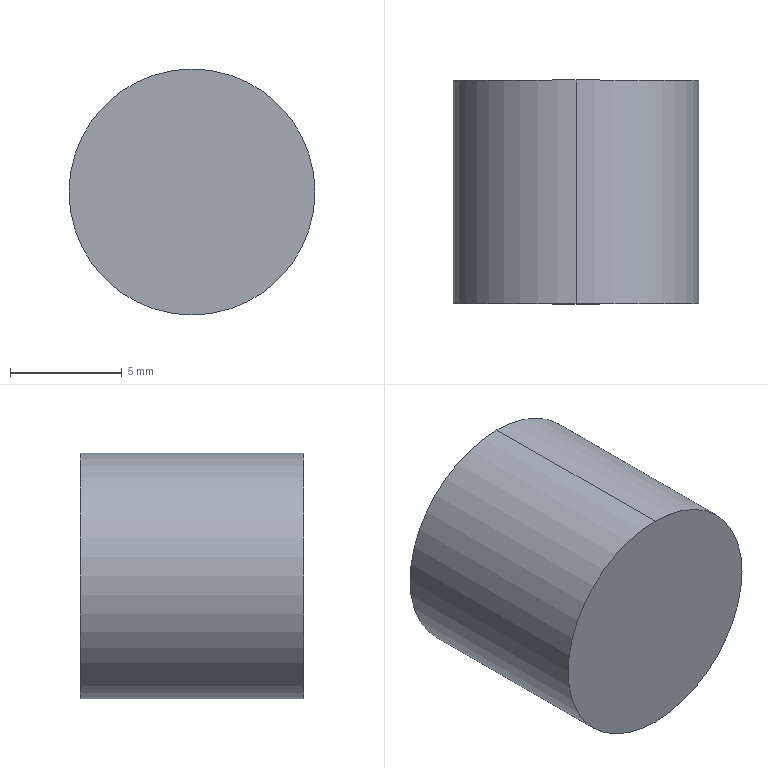Part | STEP file | OP10-129_seal pad M6 | 1 solid | 4 faces | box 11 x 10 x 11 mm | volume 950.332 mm3 | cylinder 2 | plane 2 | commonest cylinder face diameters 11 x2
STEP:
#1=CARTESIAN_POINT('',(0.,0.,0.));
#2=DIRECTION('',(0.,0.,1.));
#3=DIRECTION('',(1.,0.,0.));
#4=AXIS2_PLACEMENT_3D('',#1,#2,#3);
#5=CARTESIAN_POINT('',(0.,10.,5.5));
#6=VERTEX_POINT('',#5);
#7=CARTESIAN_POINT('',(0.,10.,-5.5));
#8=VERTEX_POINT('',#7);
#9=CARTESIAN_POINT('',(0.,10.,0.));
#10=DIRECTION('',(0.,1.,0.));
#11=DIRECTION('',(0.,0.,1.));
#12=AXIS2_PLACEMENT_3D('',#9,#10,#11);
#13=CIRCLE('',#12,5.5);
#14=CARTESIAN_POINT('',(0.,10.,0.));
#15=DIRECTION('',(0.,-1.,0.));
#16=DIRECTION('',(0.,0.,-1.));
#17=AXIS2_PLACEMENT_3D('',#14,#15,#16);
#18=CYLINDRICAL_SURFACE('',#17,5.5);
#19=CARTESIAN_POINT('',(3.142,0.));
#20=DIRECTION('',(-1.,0.));
#21=VECTOR('',#20,1.);
#22=LINE('',#19,#21);
#23=(GEOMETRIC_REPRESENTATION_CONTEXT(2)PARAMETRIC_REPRESENTATION_CONTEXT()REPRESENTATION_CONTEXT('',''));
#24=DEFINITIONAL_REPRESENTATION('',(#22),#23);
#25=PCURVE('',#18,#24);
#26=CARTESIAN_POINT('',(0.,10.,0.));
#27=DIRECTION('',(0.,1.,0.));
#28=DIRECTION('',(0.,0.,1.));
#29=AXIS2_PLACEMENT_3D('',#26,#27,#28);
#30=PLANE('',#29);
#31=CARTESIAN_POINT('',(0.,0.));
#32=DIRECTION('',(1.,0.));
#33=AXIS2_PLACEMENT_2D('',#31,#32);
#34=CIRCLE('',#33,5.5);
#35=(GEOMETRIC_REPRESENTATION_CONTEXT(2)PARAMETRIC_REPRESENTATION_CONTEXT()REPRESENTATION_CONTEXT('',''));
#36=DEFINITIONAL_REPRESENTATION('',(#34),#35);
#37=PCURVE('',#30,#36);
#38=SURFACE_CURVE('',#13,(#25,#37),.PCURVE_S1.);
#39=EDGE_CURVE('',#6,#8,#38,.T.);
#40=ORIENTED_EDGE('',*,*,#39,.F.);
#41=CARTESIAN_POINT('',(0.,0.,5.5));
#42=VERTEX_POINT('',#41);
#43=CARTESIAN_POINT('',(0.,10.,5.5));
#44=DIRECTION('',(0.,-1.,0.));
#45=VECTOR('',#44,1.);
#46=LINE('',#43,#45);
#47=CARTESIAN_POINT('',(3.142,0.));
#48=DIRECTION('',(0.,1.));
#49=VECTOR('',#48,1.);
#50=LINE('',#47,#49);
#51=(GEOMETRIC_REPRESENTATION_CONTEXT(2)PARAMETRIC_REPRESENTATION_CONTEXT()REPRESENTATION_CONTEXT('',''));
#52=DEFINITIONAL_REPRESENTATION('',(#50),#51);
#53=PCURVE('',#18,#52);
#54=CARTESIAN_POINT('',(0.,10.,0.));
#55=DIRECTION('',(0.,-1.,0.));
#56=DIRECTION('',(0.,0.,-1.));
#57=AXIS2_PLACEMENT_3D('',#54,#55,#56);
#58=CYLINDRICAL_SURFACE('',#57,5.5);
#59=CARTESIAN_POINT('',(3.142,0.));
#60=DIRECTION('',(0.,1.));
#61=VECTOR('',#60,1.);
#62=LINE('',#59,#61);
#63=(GEOMETRIC_REPRESENTATION_CONTEXT(2)PARAMETRIC_REPRESENTATION_CONTEXT()REPRESENTATION_CONTEXT('',''));
#64=DEFINITIONAL_REPRESENTATION('',(#62),#63);
#65=PCURVE('',#58,#64);
#66=SURFACE_CURVE('',#46,(#53,#65),.PCURVE_S1.);
#67=EDGE_CURVE('',#6,#42,#66,.T.);
#68=ORIENTED_EDGE('',*,*,#67,.T.);
#69=CARTESIAN_POINT('',(0.,0.,-5.5));
#70=VERTEX_POINT('',#69);
#71=CARTESIAN_POINT('',(0.,0.,0.));
#72=DIRECTION('',(0.,1.,0.));
#73=DIRECTION('',(0.,0.,1.));
#74=AXIS2_PLACEMENT_3D('',#71,#72,#73);
#75=CIRCLE('',#74,5.5);
#76=CARTESIAN_POINT('',(3.142,10.));
#77=DIRECTION('',(-1.,0.));
#78=VECTOR('',#77,1.);
#79=LINE('',#76,#78);
#80=(GEOMETRIC_REPRESENTATION_CONTEXT(2)PARAMETRIC_REPRESENTATION_CONTEXT()REPRESENTATION_CONTEXT('',''));
#81=DEFINITIONAL_REPRESENTATION('',(#79),#80);
#82=PCURVE('',#18,#81);
#83=CARTESIAN_POINT('',(0.,0.,0.));
#84=DIRECTION('',(0.,1.,0.));
#85=DIRECTION('',(0.,0.,1.));
#86=AXIS2_PLACEMENT_3D('',#83,#84,#85);
#87=PLANE('',#86);
#88=CARTESIAN_POINT('',(0.,0.));
#89=DIRECTION('',(1.,0.));
#90=AXIS2_PLACEMENT_2D('',#88,#89);
#91=CIRCLE('',#90,5.5);
#92=(GEOMETRIC_REPRESENTATION_CONTEXT(2)PARAMETRIC_REPRESENTATION_CONTEXT()REPRESENTATION_CONTEXT('',''));
#93=DEFINITIONAL_REPRESENTATION('',(#91),#92);
#94=PCURVE('',#87,#93);
#95=SURFACE_CURVE('',#75,(#82,#94),.PCURVE_S1.);
#96=EDGE_CURVE('',#42,#70,#95,.T.);
#97=ORIENTED_EDGE('',*,*,#96,.T.);
#98=CARTESIAN_POINT('',(0.,10.,-5.5));
#99=DIRECTION('',(0.,-1.,0.));
#100=VECTOR('',#99,1.);
#101=LINE('',#98,#100);
#102=CARTESIAN_POINT('',(0.,0.));
#103=DIRECTION('',(0.,1.));
#104=VECTOR('',#103,1.);
#105=LINE('',#102,#104);
#106=(GEOMETRIC_REPRESENTATION_CONTEXT(2)PARAMETRIC_REPRESENTATION_CONTEXT()REPRESENTATION_CONTEXT('',''));
#107=DEFINITIONAL_REPRESENTATION('',(#105),#106);
#108=PCURVE('',#18,#107);
#109=CARTESIAN_POINT('',(6.283,0.));
#110=DIRECTION('',(0.,1.));
#111=VECTOR('',#110,1.);
#112=LINE('',#109,#111);
#113=(GEOMETRIC_REPRESENTATION_CONTEXT(2)PARAMETRIC_REPRESENTATION_CONTEXT()REPRESENTATION_CONTEXT('',''));
#114=DEFINITIONAL_REPRESENTATION('',(#112),#113);
#115=PCURVE('',#58,#114);
#116=SURFACE_CURVE('',#101,(#108,#115),.PCURVE_S1.);
#117=EDGE_CURVE('',#8,#70,#116,.T.);
#118=ORIENTED_EDGE('',*,*,#117,.F.);
#119=EDGE_LOOP('',(#40,#68,#97,#118));
#120=FACE_BOUND('',#119,.T.);
#121=ADVANCED_FACE('',(#120),#18,.T.);
#122=ORIENTED_EDGE('',*,*,#67,.F.);
#123=CARTESIAN_POINT('',(0.,10.,0.));
#124=DIRECTION('',(0.,1.,0.));
#125=DIRECTION('',(0.,0.,1.));
#126=AXIS2_PLACEMENT_3D('',#123,#124,#125);
#127=CIRCLE('',#126,5.5);
#128=CARTESIAN_POINT('',(9.425,0.));
#129=DIRECTION('',(-1.,0.));
#130=VECTOR('',#129,1.);
#131=LINE('',#128,#130);
#132=(GEOMETRIC_REPRESENTATION_CONTEXT(2)PARAMETRIC_REPRESENTATION_CONTEXT()REPRESENTATION_CONTEXT('',''));
#133=DEFINITIONAL_REPRESENTATION('',(#131),#132);
#134=PCURVE('',#58,#133);
#135=CARTESIAN_POINT('',(0.,0.));
#136=DIRECTION('',(1.,0.));
#137=AXIS2_PLACEMENT_2D('',#135,#136);
#138=CIRCLE('',#137,5.5);
#139=(GEOMETRIC_REPRESENTATION_CONTEXT(2)PARAMETRIC_REPRESENTATION_CONTEXT()REPRESENTATION_CONTEXT('',''));
#140=DEFINITIONAL_REPRESENTATION('',(#138),#139);
#141=PCURVE('',#30,#140);
#142=SURFACE_CURVE('',#127,(#134,#141),.PCURVE_S1.);
#143=EDGE_CURVE('',#8,#6,#142,.T.);
#144=ORIENTED_EDGE('',*,*,#143,.F.);
#145=ORIENTED_EDGE('',*,*,#117,.T.);
#146=CARTESIAN_POINT('',(0.,0.,0.));
#147=DIRECTION('',(0.,1.,0.));
#148=DIRECTION('',(0.,0.,1.));
#149=AXIS2_PLACEMENT_3D('',#146,#147,#148);
#150=CIRCLE('',#149,5.5);
#151=CARTESIAN_POINT('',(9.425,10.));
#152=DIRECTION('',(-1.,0.));
#153=VECTOR('',#152,1.);
#154=LINE('',#151,#153);
#155=(GEOMETRIC_REPRESENTATION_CONTEXT(2)PARAMETRIC_REPRESENTATION_CONTEXT()REPRESENTATION_CONTEXT('',''));
#156=DEFINITIONAL_REPRESENTATION('',(#154),#155);
#157=PCURVE('',#58,#156);
#158=CARTESIAN_POINT('',(0.,0.));
#159=DIRECTION('',(1.,0.));
#160=AXIS2_PLACEMENT_2D('',#158,#159);
#161=CIRCLE('',#160,5.5);
#162=(GEOMETRIC_REPRESENTATION_CONTEXT(2)PARAMETRIC_REPRESENTATION_CONTEXT()REPRESENTATION_CONTEXT('',''));
#163=DEFINITIONAL_REPRESENTATION('',(#161),#162);
#164=PCURVE('',#87,#163);
#165=SURFACE_CURVE('',#150,(#157,#164),.PCURVE_S1.);
#166=EDGE_CURVE('',#70,#42,#165,.T.);
#167=ORIENTED_EDGE('',*,*,#166,.T.);
#168=EDGE_LOOP('',(#122,#144,#145,#167));
#169=FACE_BOUND('',#168,.T.);
#170=ADVANCED_FACE('',(#169),#58,.T.);
#171=ORIENTED_EDGE('',*,*,#143,.T.);
#172=ORIENTED_EDGE('',*,*,#39,.T.);
#173=EDGE_LOOP('',(#171,#172));
#174=FACE_BOUND('',#173,.T.);
#175=ADVANCED_FACE('',(#174),#30,.T.);
#176=ORIENTED_EDGE('',*,*,#166,.F.);
#177=ORIENTED_EDGE('',*,*,#96,.F.);
#178=EDGE_LOOP('',(#176,#177));
#179=FACE_BOUND('',#178,.T.);
#180=ADVANCED_FACE('',(#179),#87,.F.);
#181=CLOSED_SHELL('',(#121,#170,#175,#180));
#182=MANIFOLD_SOLID_BREP('',#181);
#183=(LENGTH_UNIT()NAMED_UNIT(*)SI_UNIT(.MILLI.,.METRE.));
#184=UNCERTAINTY_MEASURE_WITH_UNIT(LENGTH_MEASURE(0.0000001),#183,'','');
#185=(NAMED_UNIT(*)PLANE_ANGLE_UNIT()SI_UNIT($,.RADIAN.));
#186=(NAMED_UNIT(*)SI_UNIT($,.STERADIAN.)SOLID_ANGLE_UNIT());
#187=(GEOMETRIC_REPRESENTATION_CONTEXT(3)GLOBAL_UNCERTAINTY_ASSIGNED_CONTEXT((#184))GLOBAL_UNIT_ASSIGNED_CONTEXT((#183,#185,#186))REPRESENTATION_CONTEXT('',''));
#188=ADVANCED_BREP_SHAPE_REPRESENTATION('',(#4,#182),#187);